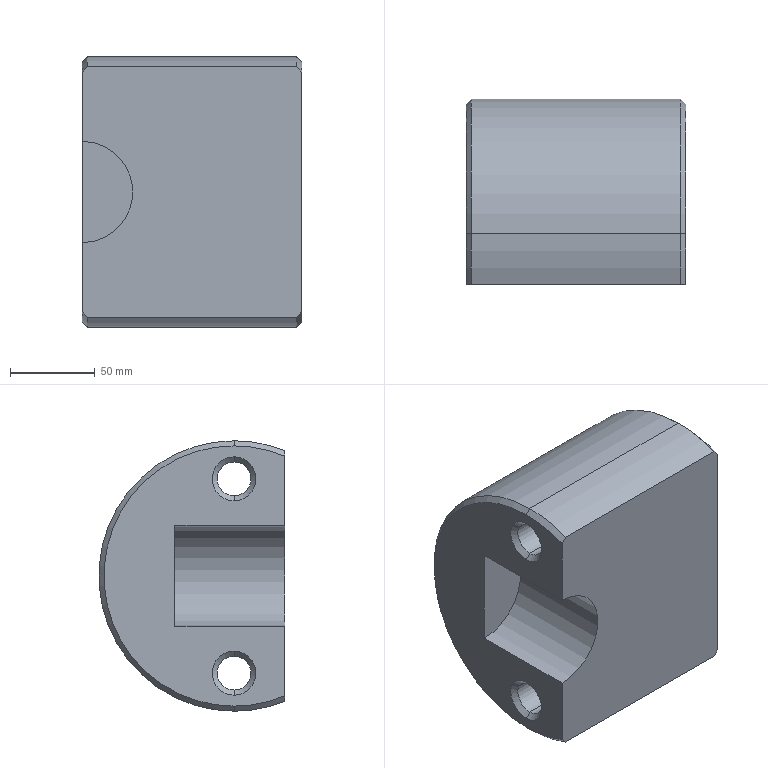Part | SolidWorks | features BaseBody 1 | 1 solid | 26 faces | box 130 x 110 x 160 mm | volume 1738348 mm3 | cone 14 | cylinder 8 | plane 4 | commonest cylinder face diameters 20 x4 160 x3 60 x1
STEP:
#1=CARTESIAN_POINT('',(240.077,228.635,230.107));
#2=VERTEX_POINT('',#1);
#3=CARTESIAN_POINT('',(240.077,228.635,290.107));
#4=VERTEX_POINT('',#3);
#5=CARTESIAN_POINT('',(240.077,228.635,260.107));
#6=DIRECTION('',(0.,-1.,0.));
#7=DIRECTION('',(0.,0.,-1.));
#8=AXIS2_PLACEMENT_3D('',#5,#6,#7);
#9=CIRCLE('',#8,30.);
#10=EDGE_CURVE('',#2,#4,#9,.T.);
#11=ORIENTED_EDGE('',*,*,#10,.F.);
#12=CARTESIAN_POINT('',(240.077,163.635,230.107));
#13=VERTEX_POINT('',#12);
#14=CARTESIAN_POINT('',(240.077,228.635,230.107));
#15=DIRECTION('',(0.,1.,0.));
#16=VECTOR('',#15,1000.);
#17=LINE('',#14,#16);
#18=EDGE_CURVE('',#13,#2,#17,.T.);
#19=ORIENTED_EDGE('',*,*,#18,.F.);
#20=CARTESIAN_POINT('',(240.077,163.635,290.107));
#21=VERTEX_POINT('',#20);
#22=CARTESIAN_POINT('',(240.077,163.635,260.107));
#23=DIRECTION('',(0.,-1.,0.));
#24=DIRECTION('',(0.,0.,-1.));
#25=AXIS2_PLACEMENT_3D('',#22,#23,#24);
#26=CIRCLE('',#25,30.);
#27=EDGE_CURVE('',#13,#21,#26,.T.);
#28=ORIENTED_EDGE('',*,*,#27,.T.);
#29=CARTESIAN_POINT('',(240.077,228.635,290.107));
#30=DIRECTION('',(0.,-1.,0.));
#31=VECTOR('',#30,1000.);
#32=LINE('',#29,#31);
#33=EDGE_CURVE('',#4,#21,#32,.T.);
#34=ORIENTED_EDGE('',*,*,#33,.F.);
#35=EDGE_LOOP('',(#11,#19,#28,#34));
#36=FACE_OUTER_BOUND('',#35,.T.);
#37=CARTESIAN_POINT('',(240.077,228.635,260.107));
#38=DIRECTION('',(0.,-1.,0.));
#39=DIRECTION('',(0.,0.,1.));
#40=AXIS2_PLACEMENT_3D('',#37,#38,#39);
#41=CYLINDRICAL_SURFACE('',#40,30.);
#42=ADVANCED_FACE('',(#36),#41,.F.);
#43=CARTESIAN_POINT('',(240.077,228.635,260.107));
#44=DIRECTION('',(0.,0.,-1.));
#45=VECTOR('',#44,1000.);
#46=LINE('',#43,#45);
#47=EDGE_CURVE('',#4,#2,#46,.T.);
#48=ORIENTED_EDGE('',*,*,#47,.T.);
#49=ORIENTED_EDGE('',*,*,#10,.T.);
#50=EDGE_LOOP('',(#48,#49));
#51=FACE_OUTER_BOUND('',#50,.T.);
#52=CARTESIAN_POINT('',(240.077,228.635,260.107));
#53=DIRECTION('',(0.,-1.,0.));
#54=DIRECTION('',(0.,0.,-1.));
#55=AXIS2_PLACEMENT_3D('',#52,#53,#54);
#56=PLANE('',#55);
#57=ADVANCED_FACE('',(#51),#56,.T.);
#58=CARTESIAN_POINT('',(240.077,193.635,337.107));
#59=VERTEX_POINT('',#58);
#60=CARTESIAN_POINT('',(243.077,193.635,340.107));
#61=VERTEX_POINT('',#60);
#62=CARTESIAN_POINT('',(243.077,193.635,340.107));
#63=DIRECTION('',(0.7071,0.,0.7071));
#64=VECTOR('',#63,1000.);
#65=LINE('',#62,#64);
#66=EDGE_CURVE('',#59,#61,#65,.T.);
#67=ORIENTED_EDGE('',*,*,#66,.F.);
#68=CARTESIAN_POINT('',(240.077,163.635,331.022));
#69=VERTEX_POINT('',#68);
#70=CARTESIAN_POINT('',(240.077,193.635,260.107));
#71=DIRECTION('',(-1.,0.,0.));
#72=DIRECTION('',(0.,0.,-1.));
#73=AXIS2_PLACEMENT_3D('',#70,#71,#72);
#74=CIRCLE('',#73,77.);
#75=EDGE_CURVE('',#69,#59,#74,.T.);
#76=ORIENTED_EDGE('',*,*,#75,.F.);
#77=CARTESIAN_POINT('',(243.077,163.635,334.269));
#78=VERTEX_POINT('',#77);
#79=CARTESIAN_POINT('',(243.077,163.635,334.269));
#80=CARTESIAN_POINT('',(242.075,163.635,333.188));
#81=CARTESIAN_POINT('',(241.075,163.635,332.106));
#82=CARTESIAN_POINT('',(240.077,163.635,331.022));
#83=B_SPLINE_CURVE_WITH_KNOTS('',3,(#79,#80,#81,#82),.UNSPECIFIED.,.F.,.F.,(4,4),(0.,1.),.UNSPECIFIED.);
#84=EDGE_CURVE('',#78,#69,#83,.T.);
#85=ORIENTED_EDGE('',*,*,#84,.F.);
#86=CARTESIAN_POINT('',(243.077,193.635,260.107));
#87=DIRECTION('',(1.,0.,0.));
#88=DIRECTION('',(0.,0.,-1.));
#89=AXIS2_PLACEMENT_3D('',#86,#87,#88);
#90=CIRCLE('',#89,80.);
#91=EDGE_CURVE('',#61,#78,#90,.T.);
#92=ORIENTED_EDGE('',*,*,#91,.F.);
#93=EDGE_LOOP('',(#67,#76,#85,#92));
#94=FACE_OUTER_BOUND('',#93,.T.);
#95=CARTESIAN_POINT('',(243.077,193.635,260.107));
#96=DIRECTION('',(1.,0.,0.));
#97=DIRECTION('',(0.,0.,1.));
#98=AXIS2_PLACEMENT_3D('',#95,#96,#97);
#99=CONICAL_SURFACE('',#98,80.,0.7854);
#100=ADVANCED_FACE('',(#94),#99,.T.);
#101=CARTESIAN_POINT('',(370.077,193.635,183.107));
#102=VERTEX_POINT('',#101);
#103=CARTESIAN_POINT('',(367.077,193.635,180.107));
#104=VERTEX_POINT('',#103);
#105=CARTESIAN_POINT('',(370.077,193.635,183.107));
#106=DIRECTION('',(-0.7071,0.,-0.7071));
#107=VECTOR('',#106,1000.);
#108=LINE('',#105,#107);
#109=EDGE_CURVE('',#102,#104,#108,.T.);
#110=ORIENTED_EDGE('',*,*,#109,.F.);
#111=CARTESIAN_POINT('',(370.077,163.635,189.191));
#112=VERTEX_POINT('',#111);
#113=CARTESIAN_POINT('',(370.077,193.635,260.107));
#114=DIRECTION('',(1.,0.,0.));
#115=DIRECTION('',(0.,0.,-1.));
#116=AXIS2_PLACEMENT_3D('',#113,#114,#115);
#117=CIRCLE('',#116,77.);
#118=EDGE_CURVE('',#112,#102,#117,.T.);
#119=ORIENTED_EDGE('',*,*,#118,.F.);
#120=CARTESIAN_POINT('',(367.077,163.635,185.945));
#121=VERTEX_POINT('',#120);
#122=CARTESIAN_POINT('',(367.077,163.635,185.945));
#123=CARTESIAN_POINT('',(368.079,163.635,187.025));
#124=CARTESIAN_POINT('',(369.079,163.635,188.107));
#125=CARTESIAN_POINT('',(370.077,163.635,189.191));
#126=B_SPLINE_CURVE_WITH_KNOTS('',3,(#122,#123,#124,#125),.UNSPECIFIED.,.F.,.F.,(4,4),(0.,1.),.UNSPECIFIED.);
#127=EDGE_CURVE('',#121,#112,#126,.T.);
#128=ORIENTED_EDGE('',*,*,#127,.F.);
#129=CARTESIAN_POINT('',(367.077,193.635,260.107));
#130=DIRECTION('',(-1.,0.,0.));
#131=DIRECTION('',(0.,0.,-1.));
#132=AXIS2_PLACEMENT_3D('',#129,#130,#131);
#133=CIRCLE('',#132,80.);
#134=EDGE_CURVE('',#104,#121,#133,.T.);
#135=ORIENTED_EDGE('',*,*,#134,.F.);
#136=EDGE_LOOP('',(#110,#119,#128,#135));
#137=FACE_OUTER_BOUND('',#136,.T.);
#138=CARTESIAN_POINT('',(370.077,193.635,260.107));
#139=DIRECTION('',(-1.,0.,0.));
#140=DIRECTION('',(0.,0.,-1.));
#141=AXIS2_PLACEMENT_3D('',#138,#139,#140);
#142=CONICAL_SURFACE('',#141,77.,0.7854);
#143=ADVANCED_FACE('',(#137),#142,.T.);
#144=CARTESIAN_POINT('',(243.077,193.635,192.607));
#145=VERTEX_POINT('',#144);
#146=CARTESIAN_POINT('',(240.077,193.635,189.607));
#147=VERTEX_POINT('',#146);
#148=CARTESIAN_POINT('',(240.077,193.635,189.607));
#149=DIRECTION('',(-0.7071,0.,-0.7071));
#150=VECTOR('',#149,1000.);
#151=LINE('',#148,#150);
#152=EDGE_CURVE('',#145,#147,#151,.T.);
#153=ORIENTED_EDGE('',*,*,#152,.F.);
#154=CARTESIAN_POINT('',(243.077,193.635,212.607));
#155=VERTEX_POINT('',#154);
#156=CARTESIAN_POINT('',(243.077,193.635,202.607));
#157=DIRECTION('',(-1.,0.,0.));
#158=DIRECTION('',(0.,0.,-1.));
#159=AXIS2_PLACEMENT_3D('',#156,#157,#158);
#160=CIRCLE('',#159,10.);
#161=EDGE_CURVE('',#155,#145,#160,.T.);
#162=ORIENTED_EDGE('',*,*,#161,.F.);
#163=CARTESIAN_POINT('',(240.077,193.635,215.607));
#164=VERTEX_POINT('',#163);
#165=CARTESIAN_POINT('',(240.077,193.635,215.607));
#166=DIRECTION('',(-0.7071,0.,0.7071));
#167=VECTOR('',#166,1000.);
#168=LINE('',#165,#167);
#169=EDGE_CURVE('',#155,#164,#168,.T.);
#170=ORIENTED_EDGE('',*,*,#169,.T.);
#171=CARTESIAN_POINT('',(240.077,193.635,202.607));
#172=DIRECTION('',(1.,0.,0.));
#173=DIRECTION('',(0.,0.,-1.));
#174=AXIS2_PLACEMENT_3D('',#171,#172,#173);
#175=CIRCLE('',#174,13.);
#176=EDGE_CURVE('',#147,#164,#175,.T.);
#177=ORIENTED_EDGE('',*,*,#176,.F.);
#178=EDGE_LOOP('',(#153,#162,#170,#177));
#179=FACE_OUTER_BOUND('',#178,.T.);
#180=CARTESIAN_POINT('',(240.077,193.635,202.607));
#181=DIRECTION('',(-1.,0.,0.));
#182=DIRECTION('',(0.,0.,-1.));
#183=AXIS2_PLACEMENT_3D('',#180,#181,#182);
#184=CONICAL_SURFACE('',#183,13.,0.7854);
#185=ADVANCED_FACE('',(#179),#184,.F.);
#186=CARTESIAN_POINT('',(243.077,193.635,307.607));
#187=VERTEX_POINT('',#186);
#188=CARTESIAN_POINT('',(240.077,193.635,304.607));
#189=VERTEX_POINT('',#188);
#190=CARTESIAN_POINT('',(240.077,193.635,304.607));
#191=DIRECTION('',(-0.7071,0.,-0.7071));
#192=VECTOR('',#191,1000.);
#193=LINE('',#190,#192);
#194=EDGE_CURVE('',#187,#189,#193,.T.);
#195=ORIENTED_EDGE('',*,*,#194,.F.);
#196=CARTESIAN_POINT('',(243.077,193.635,327.607));
#197=VERTEX_POINT('',#196);
#198=CARTESIAN_POINT('',(243.077,193.635,317.607));
#199=DIRECTION('',(-1.,0.,0.));
#200=DIRECTION('',(0.,0.,-1.));
#201=AXIS2_PLACEMENT_3D('',#198,#199,#200);
#202=CIRCLE('',#201,10.);
#203=EDGE_CURVE('',#197,#187,#202,.T.);
#204=ORIENTED_EDGE('',*,*,#203,.F.);
#205=CARTESIAN_POINT('',(240.077,193.635,330.607));
#206=VERTEX_POINT('',#205);
#207=CARTESIAN_POINT('',(240.077,193.635,330.607));
#208=DIRECTION('',(-0.7071,0.,0.7071));
#209=VECTOR('',#208,1000.);
#210=LINE('',#207,#209);
#211=EDGE_CURVE('',#197,#206,#210,.T.);
#212=ORIENTED_EDGE('',*,*,#211,.T.);
#213=CARTESIAN_POINT('',(240.077,193.635,317.607));
#214=DIRECTION('',(1.,0.,0.));
#215=DIRECTION('',(0.,0.,-1.));
#216=AXIS2_PLACEMENT_3D('',#213,#214,#215);
#217=CIRCLE('',#216,13.);
#218=EDGE_CURVE('',#189,#206,#217,.T.);
#219=ORIENTED_EDGE('',*,*,#218,.F.);
#220=EDGE_LOOP('',(#195,#204,#212,#219));
#221=FACE_OUTER_BOUND('',#220,.T.);
#222=CARTESIAN_POINT('',(240.077,193.635,317.607));
#223=DIRECTION('',(-1.,0.,0.));
#224=DIRECTION('',(0.,0.,-1.));
#225=AXIS2_PLACEMENT_3D('',#222,#223,#224);
#226=CONICAL_SURFACE('',#225,13.,0.7854);
#227=ADVANCED_FACE('',(#221),#226,.F.);
#228=CARTESIAN_POINT('',(367.077,193.635,327.607));
#229=VERTEX_POINT('',#228);
#230=CARTESIAN_POINT('',(370.077,193.635,330.607));
#231=VERTEX_POINT('',#230);
#232=CARTESIAN_POINT('',(367.077,193.635,327.607));
#233=DIRECTION('',(0.7071,0.,0.7071));
#234=VECTOR('',#233,1000.);
#235=LINE('',#232,#234);
#236=EDGE_CURVE('',#229,#231,#235,.T.);
#237=ORIENTED_EDGE('',*,*,#236,.F.);
#238=CARTESIAN_POINT('',(367.077,193.635,307.607));
#239=VERTEX_POINT('',#238);
#240=CARTESIAN_POINT('',(367.077,193.635,317.607));
#241=DIRECTION('',(1.,0.,0.));
#242=DIRECTION('',(0.,0.,-1.));
#243=AXIS2_PLACEMENT_3D('',#240,#241,#242);
#244=CIRCLE('',#243,10.);
#245=EDGE_CURVE('',#239,#229,#244,.T.);
#246=ORIENTED_EDGE('',*,*,#245,.F.);
#247=CARTESIAN_POINT('',(370.077,193.635,304.607));
#248=VERTEX_POINT('',#247);
#249=CARTESIAN_POINT('',(367.077,193.635,307.607));
#250=DIRECTION('',(0.7071,0.,-0.7071));
#251=VECTOR('',#250,1000.);
#252=LINE('',#249,#251);
#253=EDGE_CURVE('',#239,#248,#252,.T.);
#254=ORIENTED_EDGE('',*,*,#253,.T.);
#255=CARTESIAN_POINT('',(370.077,193.635,317.607));
#256=DIRECTION('',(-1.,0.,0.));
#257=DIRECTION('',(0.,0.,-1.));
#258=AXIS2_PLACEMENT_3D('',#255,#256,#257);
#259=CIRCLE('',#258,13.);
#260=EDGE_CURVE('',#231,#248,#259,.T.);
#261=ORIENTED_EDGE('',*,*,#260,.F.);
#262=EDGE_LOOP('',(#237,#246,#254,#261));
#263=FACE_OUTER_BOUND('',#262,.T.);
#264=CARTESIAN_POINT('',(367.077,193.635,317.607));
#265=DIRECTION('',(1.,0.,0.));
#266=DIRECTION('',(0.,0.,1.));
#267=AXIS2_PLACEMENT_3D('',#264,#265,#266);
#268=CONICAL_SURFACE('',#267,10.,0.7854);
#269=ADVANCED_FACE('',(#263),#268,.F.);
#270=CARTESIAN_POINT('',(367.077,193.635,212.607));
#271=VERTEX_POINT('',#270);
#272=CARTESIAN_POINT('',(370.077,193.635,215.607));
#273=VERTEX_POINT('',#272);
#274=CARTESIAN_POINT('',(367.077,193.635,212.607));
#275=DIRECTION('',(0.7071,0.,0.7071));
#276=VECTOR('',#275,1000.);
#277=LINE('',#274,#276);
#278=EDGE_CURVE('',#271,#273,#277,.T.);
#279=ORIENTED_EDGE('',*,*,#278,.F.);
#280=CARTESIAN_POINT('',(367.077,193.635,192.607));
#281=VERTEX_POINT('',#280);
#282=CARTESIAN_POINT('',(367.077,193.635,202.607));
#283=DIRECTION('',(1.,0.,0.));
#284=DIRECTION('',(0.,0.,-1.));
#285=AXIS2_PLACEMENT_3D('',#282,#283,#284);
#286=CIRCLE('',#285,10.);
#287=EDGE_CURVE('',#281,#271,#286,.T.);
#288=ORIENTED_EDGE('',*,*,#287,.F.);
#289=CARTESIAN_POINT('',(370.077,193.635,189.607));
#290=VERTEX_POINT('',#289);
#291=CARTESIAN_POINT('',(367.077,193.635,192.607));
#292=DIRECTION('',(0.7071,0.,-0.7071));
#293=VECTOR('',#292,1000.);
#294=LINE('',#291,#293);
#295=EDGE_CURVE('',#281,#290,#294,.T.);
#296=ORIENTED_EDGE('',*,*,#295,.T.);
#297=CARTESIAN_POINT('',(370.077,193.635,202.607));
#298=DIRECTION('',(-1.,0.,0.));
#299=DIRECTION('',(0.,0.,-1.));
#300=AXIS2_PLACEMENT_3D('',#297,#298,#299);
#301=CIRCLE('',#300,13.);
#302=EDGE_CURVE('',#273,#290,#301,.T.);
#303=ORIENTED_EDGE('',*,*,#302,.F.);
#304=EDGE_LOOP('',(#279,#288,#296,#303));
#305=FACE_OUTER_BOUND('',#304,.T.);
#306=CARTESIAN_POINT('',(367.077,193.635,202.607));
#307=DIRECTION('',(1.,0.,0.));
#308=DIRECTION('',(0.,0.,1.));
#309=AXIS2_PLACEMENT_3D('',#306,#307,#308);
#310=CONICAL_SURFACE('',#309,10.,0.7854);
#311=ADVANCED_FACE('',(#305),#310,.F.);
#312=CARTESIAN_POINT('',(370.077,193.635,192.607));
#313=DIRECTION('',(-1.,0.,0.));
#314=VECTOR('',#313,1000.);
#315=LINE('',#312,#314);
#316=EDGE_CURVE('',#281,#145,#315,.T.);
#317=ORIENTED_EDGE('',*,*,#316,.F.);
#318=ORIENTED_EDGE('',*,*,#287,.T.);
#319=CARTESIAN_POINT('',(370.077,193.635,212.607));
#320=DIRECTION('',(-1.,0.,0.));
#321=VECTOR('',#320,1000.);
#322=LINE('',#319,#321);
#323=EDGE_CURVE('',#271,#155,#322,.T.);
#324=ORIENTED_EDGE('',*,*,#323,.T.);
#325=ORIENTED_EDGE('',*,*,#161,.T.);
#326=EDGE_LOOP('',(#317,#318,#324,#325));
#327=FACE_OUTER_BOUND('',#326,.T.);
#328=CARTESIAN_POINT('',(370.077,193.635,202.607));
#329=DIRECTION('',(-1.,0.,0.));
#330=DIRECTION('',(0.,0.,-1.));
#331=AXIS2_PLACEMENT_3D('',#328,#329,#330);
#332=CYLINDRICAL_SURFACE('',#331,10.);
#333=ADVANCED_FACE('',(#327),#332,.F.);
#334=CARTESIAN_POINT('',(370.077,193.635,307.607));
#335=DIRECTION('',(-1.,0.,0.));
#336=VECTOR('',#335,1000.);
#337=LINE('',#334,#336);
#338=EDGE_CURVE('',#239,#187,#337,.T.);
#339=ORIENTED_EDGE('',*,*,#338,.F.);
#340=ORIENTED_EDGE('',*,*,#245,.T.);
#341=CARTESIAN_POINT('',(370.077,193.635,327.607));
#342=DIRECTION('',(-1.,0.,0.));
#343=VECTOR('',#342,1000.);
#344=LINE('',#341,#343);
#345=EDGE_CURVE('',#229,#197,#344,.T.);
#346=ORIENTED_EDGE('',*,*,#345,.T.);
#347=ORIENTED_EDGE('',*,*,#203,.T.);
#348=EDGE_LOOP('',(#339,#340,#346,#347));
#349=FACE_OUTER_BOUND('',#348,.T.);
#350=CARTESIAN_POINT('',(370.077,193.635,317.607));
#351=DIRECTION('',(-1.,0.,0.));
#352=DIRECTION('',(0.,0.,-1.));
#353=AXIS2_PLACEMENT_3D('',#350,#351,#352);
#354=CYLINDRICAL_SURFACE('',#353,10.);
#355=ADVANCED_FACE('',(#349),#354,.F.);
#356=CARTESIAN_POINT('',(240.077,163.635,260.107));
#357=DIRECTION('',(0.,0.,-1.));
#358=VECTOR('',#357,1000.);
#359=LINE('',#356,#358);
#360=EDGE_CURVE('',#69,#21,#359,.T.);
#361=ORIENTED_EDGE('',*,*,#360,.T.);
#362=ORIENTED_EDGE('',*,*,#27,.F.);
#363=CARTESIAN_POINT('',(240.077,163.635,189.191));
#364=VERTEX_POINT('',#363);
#365=CARTESIAN_POINT('',(240.077,163.635,260.107));
#366=DIRECTION('',(0.,0.,-1.));
#367=VECTOR('',#366,1000.);
#368=LINE('',#365,#367);
#369=EDGE_CURVE('',#13,#364,#368,.T.);
#370=ORIENTED_EDGE('',*,*,#369,.T.);
#371=CARTESIAN_POINT('',(243.077,163.635,185.945));
#372=VERTEX_POINT('',#371);
#373=CARTESIAN_POINT('',(240.077,163.635,189.191));
#374=CARTESIAN_POINT('',(241.075,163.635,188.107));
#375=CARTESIAN_POINT('',(242.075,163.635,187.025));
#376=CARTESIAN_POINT('',(243.077,163.635,185.945));
#377=B_SPLINE_CURVE_WITH_KNOTS('',3,(#373,#374,#375,#376),.UNSPECIFIED.,.F.,.F.,(4,4),(0.,1.),.UNSPECIFIED.);
#378=EDGE_CURVE('',#364,#372,#377,.T.);
#379=ORIENTED_EDGE('',*,*,#378,.T.);
#380=CARTESIAN_POINT('',(370.077,163.635,185.945));
#381=DIRECTION('',(-1.,0.,0.));
#382=VECTOR('',#381,1000.);
#383=LINE('',#380,#382);
#384=EDGE_CURVE('',#121,#372,#383,.T.);
#385=ORIENTED_EDGE('',*,*,#384,.F.);
#386=ORIENTED_EDGE('',*,*,#127,.T.);
#387=CARTESIAN_POINT('',(370.077,163.635,331.022));
#388=VERTEX_POINT('',#387);
#389=CARTESIAN_POINT('',(370.077,163.635,260.107));
#390=DIRECTION('',(0.,0.,-1.));
#391=VECTOR('',#390,1000.);
#392=LINE('',#389,#391);
#393=EDGE_CURVE('',#388,#112,#392,.T.);
#394=ORIENTED_EDGE('',*,*,#393,.F.);
#395=CARTESIAN_POINT('',(367.077,163.635,334.269));
#396=VERTEX_POINT('',#395);
#397=CARTESIAN_POINT('',(370.077,163.635,331.022));
#398=CARTESIAN_POINT('',(369.079,163.635,332.106));
#399=CARTESIAN_POINT('',(368.079,163.635,333.188));
#400=CARTESIAN_POINT('',(367.077,163.635,334.269));
#401=B_SPLINE_CURVE_WITH_KNOTS('',3,(#397,#398,#399,#400),.UNSPECIFIED.,.F.,.F.,(4,4),(0.,1.),.UNSPECIFIED.);
#402=EDGE_CURVE('',#388,#396,#401,.T.);
#403=ORIENTED_EDGE('',*,*,#402,.T.);
#404=CARTESIAN_POINT('',(370.077,163.635,334.269));
#405=DIRECTION('',(-1.,0.,0.));
#406=VECTOR('',#405,1000.);
#407=LINE('',#404,#406);
#408=EDGE_CURVE('',#396,#78,#407,.T.);
#409=ORIENTED_EDGE('',*,*,#408,.T.);
#410=ORIENTED_EDGE('',*,*,#84,.T.);
#411=EDGE_LOOP('',(#361,#362,#370,#379,#385,#386,#394,#403,#409,#410));
#412=FACE_OUTER_BOUND('',#411,.T.);
#413=CARTESIAN_POINT('',(370.077,163.635,260.107));
#414=DIRECTION('',(0.,1.,0.));
#415=DIRECTION('',(1.,0.,0.));
#416=AXIS2_PLACEMENT_3D('',#413,#414,#415);
#417=PLANE('',#416);
#418=ADVANCED_FACE('',(#412),#417,.F.);
#419=CARTESIAN_POINT('',(243.077,193.635,180.107));
#420=VERTEX_POINT('',#419);
#421=CARTESIAN_POINT('',(370.077,193.635,180.107));
#422=DIRECTION('',(-1.,0.,0.));
#423=VECTOR('',#422,1000.);
#424=LINE('',#421,#423);
#425=EDGE_CURVE('',#104,#420,#424,.T.);
#426=ORIENTED_EDGE('',*,*,#425,.F.);
#427=ORIENTED_EDGE('',*,*,#134,.T.);
#428=ORIENTED_EDGE('',*,*,#384,.T.);
#429=CARTESIAN_POINT('',(243.077,193.635,260.107));
#430=DIRECTION('',(1.,0.,0.));
#431=DIRECTION('',(0.,0.,-1.));
#432=AXIS2_PLACEMENT_3D('',#429,#430,#431);
#433=CIRCLE('',#432,80.);
#434=EDGE_CURVE('',#372,#420,#433,.T.);
#435=ORIENTED_EDGE('',*,*,#434,.T.);
#436=EDGE_LOOP('',(#426,#427,#428,#435));
#437=FACE_OUTER_BOUND('',#436,.T.);
#438=CARTESIAN_POINT('',(370.077,193.635,260.107));
#439=DIRECTION('',(-1.,0.,0.));
#440=DIRECTION('',(0.,0.,-1.));
#441=AXIS2_PLACEMENT_3D('',#438,#439,#440);
#442=CYLINDRICAL_SURFACE('',#441,80.);
#443=ADVANCED_FACE('',(#437),#442,.T.);
#444=CARTESIAN_POINT('',(240.077,193.635,202.607));
#445=DIRECTION('',(1.,0.,0.));
#446=DIRECTION('',(0.,0.,-1.));
#447=AXIS2_PLACEMENT_3D('',#444,#445,#446);
#448=CIRCLE('',#447,13.);
#449=EDGE_CURVE('',#164,#147,#448,.T.);
#450=ORIENTED_EDGE('',*,*,#449,.T.);
#451=ORIENTED_EDGE('',*,*,#176,.T.);
#452=EDGE_LOOP('',(#450,#451));
#453=FACE_BOUND('',#452,.T.);
#454=CARTESIAN_POINT('',(240.077,193.635,317.607));
#455=DIRECTION('',(1.,0.,0.));
#456=DIRECTION('',(0.,0.,-1.));
#457=AXIS2_PLACEMENT_3D('',#454,#455,#456);
#458=CIRCLE('',#457,13.);
#459=EDGE_CURVE('',#206,#189,#458,.T.);
#460=ORIENTED_EDGE('',*,*,#459,.T.);
#461=ORIENTED_EDGE('',*,*,#218,.T.);
#462=EDGE_LOOP('',(#460,#461));
#463=FACE_BOUND('',#462,.T.);
#464=ORIENTED_EDGE('',*,*,#47,.F.);
#465=ORIENTED_EDGE('',*,*,#33,.T.);
#466=ORIENTED_EDGE('',*,*,#360,.F.);
#467=ORIENTED_EDGE('',*,*,#75,.T.);
#468=CARTESIAN_POINT('',(240.077,193.635,183.107));
#469=VERTEX_POINT('',#468);
#470=CARTESIAN_POINT('',(240.077,193.635,260.107));
#471=DIRECTION('',(-1.,0.,0.));
#472=DIRECTION('',(0.,0.,-1.));
#473=AXIS2_PLACEMENT_3D('',#470,#471,#472);
#474=CIRCLE('',#473,77.);
#475=EDGE_CURVE('',#59,#469,#474,.T.);
#476=ORIENTED_EDGE('',*,*,#475,.T.);
#477=CARTESIAN_POINT('',(240.077,193.635,260.107));
#478=DIRECTION('',(-1.,0.,0.));
#479=DIRECTION('',(0.,0.,-1.));
#480=AXIS2_PLACEMENT_3D('',#477,#478,#479);
#481=CIRCLE('',#480,77.);
#482=EDGE_CURVE('',#469,#364,#481,.T.);
#483=ORIENTED_EDGE('',*,*,#482,.T.);
#484=ORIENTED_EDGE('',*,*,#369,.F.);
#485=ORIENTED_EDGE('',*,*,#18,.T.);
#486=EDGE_LOOP('',(#464,#465,#466,#467,#476,#483,#484,#485));
#487=FACE_OUTER_BOUND('',#486,.T.);
#488=CARTESIAN_POINT('',(240.077,193.635,260.107));
#489=DIRECTION('',(1.,0.,0.));
#490=DIRECTION('',(0.,1.,0.));
#491=AXIS2_PLACEMENT_3D('',#488,#489,#490);
#492=PLANE('',#491);
#493=ADVANCED_FACE('',(#453,#463,#487),#492,.F.);
#494=CARTESIAN_POINT('',(370.077,193.635,317.607));
#495=DIRECTION('',(-1.,0.,0.));
#496=DIRECTION('',(0.,0.,-1.));
#497=AXIS2_PLACEMENT_3D('',#494,#495,#496);
#498=CIRCLE('',#497,13.);
#499=EDGE_CURVE('',#248,#231,#498,.T.);
#500=ORIENTED_EDGE('',*,*,#499,.T.);
#501=ORIENTED_EDGE('',*,*,#260,.T.);
#502=EDGE_LOOP('',(#500,#501));
#503=FACE_BOUND('',#502,.T.);
#504=CARTESIAN_POINT('',(370.077,193.635,202.607));
#505=DIRECTION('',(-1.,0.,0.));
#506=DIRECTION('',(0.,0.,-1.));
#507=AXIS2_PLACEMENT_3D('',#504,#505,#506);
#508=CIRCLE('',#507,13.);
#509=EDGE_CURVE('',#290,#273,#508,.T.);
#510=ORIENTED_EDGE('',*,*,#509,.T.);
#511=ORIENTED_EDGE('',*,*,#302,.T.);
#512=EDGE_LOOP('',(#510,#511));
#513=FACE_BOUND('',#512,.T.);
#514=ORIENTED_EDGE('',*,*,#393,.T.);
#515=ORIENTED_EDGE('',*,*,#118,.T.);
#516=CARTESIAN_POINT('',(370.077,193.635,337.107));
#517=VERTEX_POINT('',#516);
#518=CARTESIAN_POINT('',(370.077,193.635,260.107));
#519=DIRECTION('',(1.,0.,0.));
#520=DIRECTION('',(0.,0.,-1.));
#521=AXIS2_PLACEMENT_3D('',#518,#519,#520);
#522=CIRCLE('',#521,77.);
#523=EDGE_CURVE('',#102,#517,#522,.T.);
#524=ORIENTED_EDGE('',*,*,#523,.T.);
#525=CARTESIAN_POINT('',(370.077,193.635,260.107));
#526=DIRECTION('',(1.,0.,0.));
#527=DIRECTION('',(0.,0.,-1.));
#528=AXIS2_PLACEMENT_3D('',#525,#526,#527);
#529=CIRCLE('',#528,77.);
#530=EDGE_CURVE('',#517,#388,#529,.T.);
#531=ORIENTED_EDGE('',*,*,#530,.T.);
#532=EDGE_LOOP('',(#514,#515,#524,#531));
#533=FACE_OUTER_BOUND('',#532,.T.);
#534=CARTESIAN_POINT('',(370.077,193.635,260.107));
#535=DIRECTION('',(1.,0.,0.));
#536=DIRECTION('',(0.,1.,0.));
#537=AXIS2_PLACEMENT_3D('',#534,#535,#536);
#538=PLANE('',#537);
#539=ADVANCED_FACE('',(#503,#513,#533),#538,.T.);
#540=CARTESIAN_POINT('',(367.077,193.635,340.107));
#541=VERTEX_POINT('',#540);
#542=CARTESIAN_POINT('',(367.077,193.635,260.107));
#543=DIRECTION('',(-1.,0.,0.));
#544=DIRECTION('',(0.,0.,-1.));
#545=AXIS2_PLACEMENT_3D('',#542,#543,#544);
#546=CIRCLE('',#545,80.);
#547=EDGE_CURVE('',#396,#541,#546,.T.);
#548=ORIENTED_EDGE('',*,*,#547,.T.);
#549=CARTESIAN_POINT('',(370.077,193.635,340.107));
#550=DIRECTION('',(-1.,0.,0.));
#551=VECTOR('',#550,1000.);
#552=LINE('',#549,#551);
#553=EDGE_CURVE('',#541,#61,#552,.T.);
#554=ORIENTED_EDGE('',*,*,#553,.T.);
#555=ORIENTED_EDGE('',*,*,#91,.T.);
#556=ORIENTED_EDGE('',*,*,#408,.F.);
#557=EDGE_LOOP('',(#548,#554,#555,#556));
#558=FACE_OUTER_BOUND('',#557,.T.);
#559=CARTESIAN_POINT('',(370.077,193.635,260.107));
#560=DIRECTION('',(-1.,0.,0.));
#561=DIRECTION('',(0.,0.,-1.));
#562=AXIS2_PLACEMENT_3D('',#559,#560,#561);
#563=CYLINDRICAL_SURFACE('',#562,80.);
#564=ADVANCED_FACE('',(#558),#563,.T.);
#565=CARTESIAN_POINT('',(367.077,193.635,260.107));
#566=DIRECTION('',(-1.,0.,0.));
#567=DIRECTION('',(0.,0.,-1.));
#568=AXIS2_PLACEMENT_3D('',#565,#566,#567);
#569=CIRCLE('',#568,80.);
#570=EDGE_CURVE('',#541,#104,#569,.T.);
#571=ORIENTED_EDGE('',*,*,#570,.T.);
#572=ORIENTED_EDGE('',*,*,#425,.T.);
#573=CARTESIAN_POINT('',(243.077,193.635,260.107));
#574=DIRECTION('',(1.,0.,0.));
#575=DIRECTION('',(0.,0.,-1.));
#576=AXIS2_PLACEMENT_3D('',#573,#574,#575);
#577=CIRCLE('',#576,80.);
#578=EDGE_CURVE('',#420,#61,#577,.T.);
#579=ORIENTED_EDGE('',*,*,#578,.T.);
#580=ORIENTED_EDGE('',*,*,#553,.F.);
#581=EDGE_LOOP('',(#571,#572,#579,#580));
#582=FACE_OUTER_BOUND('',#581,.T.);
#583=CARTESIAN_POINT('',(370.077,193.635,260.107));
#584=DIRECTION('',(-1.,0.,0.));
#585=DIRECTION('',(0.,0.,-1.));
#586=AXIS2_PLACEMENT_3D('',#583,#584,#585);
#587=CYLINDRICAL_SURFACE('',#586,80.);
#588=ADVANCED_FACE('',(#582),#587,.T.);
#589=CARTESIAN_POINT('',(367.077,193.635,317.607));
#590=DIRECTION('',(1.,0.,0.));
#591=DIRECTION('',(0.,0.,-1.));
#592=AXIS2_PLACEMENT_3D('',#589,#590,#591);
#593=CIRCLE('',#592,10.);
#594=EDGE_CURVE('',#229,#239,#593,.T.);
#595=ORIENTED_EDGE('',*,*,#594,.T.);
#596=ORIENTED_EDGE('',*,*,#338,.T.);
#597=CARTESIAN_POINT('',(243.077,193.635,317.607));
#598=DIRECTION('',(-1.,0.,0.));
#599=DIRECTION('',(0.,0.,-1.));
#600=AXIS2_PLACEMENT_3D('',#597,#598,#599);
#601=CIRCLE('',#600,10.);
#602=EDGE_CURVE('',#187,#197,#601,.T.);
#603=ORIENTED_EDGE('',*,*,#602,.T.);
#604=ORIENTED_EDGE('',*,*,#345,.F.);
#605=EDGE_LOOP('',(#595,#596,#603,#604));
#606=FACE_OUTER_BOUND('',#605,.T.);
#607=CARTESIAN_POINT('',(370.077,193.635,317.607));
#608=DIRECTION('',(-1.,0.,0.));
#609=DIRECTION('',(0.,0.,-1.));
#610=AXIS2_PLACEMENT_3D('',#607,#608,#609);
#611=CYLINDRICAL_SURFACE('',#610,10.);
#612=ADVANCED_FACE('',(#606),#611,.F.);
#613=CARTESIAN_POINT('',(367.077,193.635,202.607));
#614=DIRECTION('',(1.,0.,0.));
#615=DIRECTION('',(0.,0.,-1.));
#616=AXIS2_PLACEMENT_3D('',#613,#614,#615);
#617=CIRCLE('',#616,10.);
#618=EDGE_CURVE('',#271,#281,#617,.T.);
#619=ORIENTED_EDGE('',*,*,#618,.T.);
#620=ORIENTED_EDGE('',*,*,#316,.T.);
#621=CARTESIAN_POINT('',(243.077,193.635,202.607));
#622=DIRECTION('',(-1.,0.,0.));
#623=DIRECTION('',(0.,0.,-1.));
#624=AXIS2_PLACEMENT_3D('',#621,#622,#623);
#625=CIRCLE('',#624,10.);
#626=EDGE_CURVE('',#145,#155,#625,.T.);
#627=ORIENTED_EDGE('',*,*,#626,.T.);
#628=ORIENTED_EDGE('',*,*,#323,.F.);
#629=EDGE_LOOP('',(#619,#620,#627,#628));
#630=FACE_OUTER_BOUND('',#629,.T.);
#631=CARTESIAN_POINT('',(370.077,193.635,202.607));
#632=DIRECTION('',(-1.,0.,0.));
#633=DIRECTION('',(0.,0.,-1.));
#634=AXIS2_PLACEMENT_3D('',#631,#632,#633);
#635=CYLINDRICAL_SURFACE('',#634,10.);
#636=ADVANCED_FACE('',(#630),#635,.F.);
#637=ORIENTED_EDGE('',*,*,#618,.F.);
#638=ORIENTED_EDGE('',*,*,#278,.T.);
#639=ORIENTED_EDGE('',*,*,#509,.F.);
#640=ORIENTED_EDGE('',*,*,#295,.F.);
#641=EDGE_LOOP('',(#637,#638,#639,#640));
#642=FACE_OUTER_BOUND('',#641,.T.);
#643=CARTESIAN_POINT('',(367.077,193.635,202.607));
#644=DIRECTION('',(1.,0.,0.));
#645=DIRECTION('',(0.,0.,1.));
#646=AXIS2_PLACEMENT_3D('',#643,#644,#645);
#647=CONICAL_SURFACE('',#646,10.,0.7854);
#648=ADVANCED_FACE('',(#642),#647,.F.);
#649=ORIENTED_EDGE('',*,*,#594,.F.);
#650=ORIENTED_EDGE('',*,*,#236,.T.);
#651=ORIENTED_EDGE('',*,*,#499,.F.);
#652=ORIENTED_EDGE('',*,*,#253,.F.);
#653=EDGE_LOOP('',(#649,#650,#651,#652));
#654=FACE_OUTER_BOUND('',#653,.T.);
#655=CARTESIAN_POINT('',(367.077,193.635,317.607));
#656=DIRECTION('',(1.,0.,0.));
#657=DIRECTION('',(0.,0.,1.));
#658=AXIS2_PLACEMENT_3D('',#655,#656,#657);
#659=CONICAL_SURFACE('',#658,10.,0.7854);
#660=ADVANCED_FACE('',(#654),#659,.F.);
#661=ORIENTED_EDGE('',*,*,#602,.F.);
#662=ORIENTED_EDGE('',*,*,#194,.T.);
#663=ORIENTED_EDGE('',*,*,#459,.F.);
#664=ORIENTED_EDGE('',*,*,#211,.F.);
#665=EDGE_LOOP('',(#661,#662,#663,#664));
#666=FACE_OUTER_BOUND('',#665,.T.);
#667=CARTESIAN_POINT('',(240.077,193.635,317.607));
#668=DIRECTION('',(-1.,0.,0.));
#669=DIRECTION('',(0.,0.,-1.));
#670=AXIS2_PLACEMENT_3D('',#667,#668,#669);
#671=CONICAL_SURFACE('',#670,13.,0.7854);
#672=ADVANCED_FACE('',(#666),#671,.F.);
#673=ORIENTED_EDGE('',*,*,#626,.F.);
#674=ORIENTED_EDGE('',*,*,#152,.T.);
#675=ORIENTED_EDGE('',*,*,#449,.F.);
#676=ORIENTED_EDGE('',*,*,#169,.F.);
#677=EDGE_LOOP('',(#673,#674,#675,#676));
#678=FACE_OUTER_BOUND('',#677,.T.);
#679=CARTESIAN_POINT('',(240.077,193.635,202.607));
#680=DIRECTION('',(-1.,0.,0.));
#681=DIRECTION('',(0.,0.,-1.));
#682=AXIS2_PLACEMENT_3D('',#679,#680,#681);
#683=CONICAL_SURFACE('',#682,13.,0.7854);
#684=ADVANCED_FACE('',(#678),#683,.F.);
#685=ORIENTED_EDGE('',*,*,#530,.F.);
#686=CARTESIAN_POINT('',(370.077,193.635,337.107));
#687=DIRECTION('',(-0.7071,0.,0.7071));
#688=VECTOR('',#687,1000.);
#689=LINE('',#686,#688);
#690=EDGE_CURVE('',#517,#541,#689,.T.);
#691=ORIENTED_EDGE('',*,*,#690,.T.);
#692=ORIENTED_EDGE('',*,*,#547,.F.);
#693=ORIENTED_EDGE('',*,*,#402,.F.);
#694=EDGE_LOOP('',(#685,#691,#692,#693));
#695=FACE_OUTER_BOUND('',#694,.T.);
#696=CARTESIAN_POINT('',(370.077,193.635,260.107));
#697=DIRECTION('',(-1.,0.,0.));
#698=DIRECTION('',(0.,0.,-1.));
#699=AXIS2_PLACEMENT_3D('',#696,#697,#698);
#700=CONICAL_SURFACE('',#699,77.,0.7854);
#701=ADVANCED_FACE('',(#695),#700,.T.);
#702=ORIENTED_EDGE('',*,*,#523,.F.);
#703=ORIENTED_EDGE('',*,*,#109,.T.);
#704=ORIENTED_EDGE('',*,*,#570,.F.);
#705=ORIENTED_EDGE('',*,*,#690,.F.);
#706=EDGE_LOOP('',(#702,#703,#704,#705));
#707=FACE_OUTER_BOUND('',#706,.T.);
#708=CARTESIAN_POINT('',(370.077,193.635,260.107));
#709=DIRECTION('',(-1.,0.,0.));
#710=DIRECTION('',(0.,0.,-1.));
#711=AXIS2_PLACEMENT_3D('',#708,#709,#710);
#712=CONICAL_SURFACE('',#711,77.,0.7854);
#713=ADVANCED_FACE('',(#707),#712,.T.);
#714=ORIENTED_EDGE('',*,*,#482,.F.);
#715=CARTESIAN_POINT('',(243.077,193.635,180.107));
#716=DIRECTION('',(0.7071,0.,-0.7071));
#717=VECTOR('',#716,1000.);
#718=LINE('',#715,#717);
#719=EDGE_CURVE('',#469,#420,#718,.T.);
#720=ORIENTED_EDGE('',*,*,#719,.T.);
#721=ORIENTED_EDGE('',*,*,#434,.F.);
#722=ORIENTED_EDGE('',*,*,#378,.F.);
#723=EDGE_LOOP('',(#714,#720,#721,#722));
#724=FACE_OUTER_BOUND('',#723,.T.);
#725=CARTESIAN_POINT('',(243.077,193.635,260.107));
#726=DIRECTION('',(1.,0.,0.));
#727=DIRECTION('',(0.,0.,1.));
#728=AXIS2_PLACEMENT_3D('',#725,#726,#727);
#729=CONICAL_SURFACE('',#728,80.,0.7854);
#730=ADVANCED_FACE('',(#724),#729,.T.);
#731=ORIENTED_EDGE('',*,*,#475,.F.);
#732=ORIENTED_EDGE('',*,*,#66,.T.);
#733=ORIENTED_EDGE('',*,*,#578,.F.);
#734=ORIENTED_EDGE('',*,*,#719,.F.);
#735=EDGE_LOOP('',(#731,#732,#733,#734));
#736=FACE_OUTER_BOUND('',#735,.T.);
#737=CARTESIAN_POINT('',(243.077,193.635,260.107));
#738=DIRECTION('',(1.,0.,0.));
#739=DIRECTION('',(0.,0.,1.));
#740=AXIS2_PLACEMENT_3D('',#737,#738,#739);
#741=CONICAL_SURFACE('',#740,80.,0.7854);
#742=ADVANCED_FACE('',(#736),#741,.T.);
#743=CLOSED_SHELL('',(#42,#57,#100,#143,#185,#227,#269,#311,#333,#355,#418,#443,#493,#539,#564,#588,#612,#636,#648,#660,#672,#684,#701,#713,#730,#742));
#744=MANIFOLD_SOLID_BREP('',#743);
#745=CARTESIAN_POINT('',(0.,0.,0.));
#746=DIRECTION('',(0.,0.,1.));
#747=DIRECTION('',(1.,0.,0.));
#748=AXIS2_PLACEMENT_3D('',#745,#746,#747);
#749=(LENGTH_UNIT()NAMED_UNIT(*)SI_UNIT(.MILLI.,.METRE.));
#750=UNCERTAINTY_MEASURE_WITH_UNIT(LENGTH_MEASURE(0.00001),#749,'','');
#751=(NAMED_UNIT(*)PLANE_ANGLE_UNIT()SI_UNIT($,.RADIAN.));
#752=(NAMED_UNIT(*)SI_UNIT($,.STERADIAN.)SOLID_ANGLE_UNIT());
#753=(GEOMETRIC_REPRESENTATION_CONTEXT(3)GLOBAL_UNCERTAINTY_ASSIGNED_CONTEXT((#750))GLOBAL_UNIT_ASSIGNED_CONTEXT((#749,#751,#752))REPRESENTATION_CONTEXT('',''));
#754=ADVANCED_BREP_SHAPE_REPRESENTATION('',(#744,#748),#753);